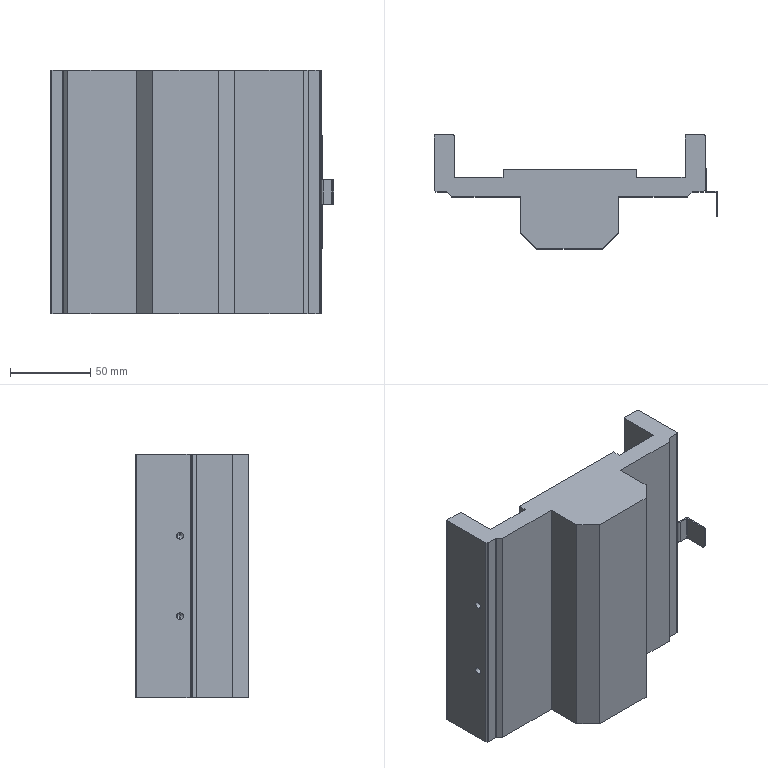Part | STEP file | Single-axis manipulator CFS17-L10-650-BR-T750-C4-MB-3M-slider | 2 solids | 124 faces | box 177 x 71 x 152 mm | volume 741184 mm3 | cylinder 52 | plane 44 | cone 28 | commonest cylinder face diameters 6.8 x16 1 x12 4.2 x8 2 x6 5.6 x4 6 x4